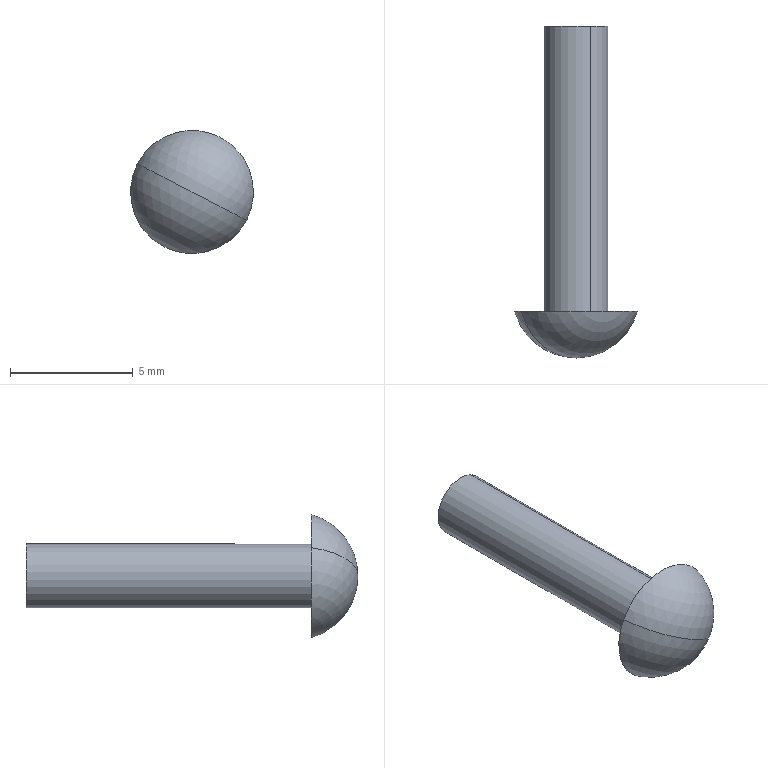Part | SolidWorks | features BaseBody 1 | 1 solid | 6 faces | box 5 x 13.501 x 5 mm | volume 83.832 mm3 | sphere 2 | plane 2 | cylinder 2 | commonest cylinder face diameters 2.6 x2
STEP:
#1=CARTESIAN_POINT('',(-214.693,5.922,3.237));
#2=VERTEX_POINT('',#1);
#3=CARTESIAN_POINT('',(-210.253,5.923,0.9371));
#4=VERTEX_POINT('',#3);
#5=CARTESIAN_POINT('',(-212.473,6.618,2.087));
#6=DIRECTION('',(0.46,-0.0003779,0.8879));
#7=DIRECTION('',(0.00003827,-1.,-0.0004455));
#8=AXIS2_PLACEMENT_3D('',#5,#6,#7);
#9=CIRCLE('',#8,2.595);
#10=EDGE_CURVE('',#2,#4,#9,.T.);
#11=ORIENTED_EDGE('',*,*,#10,.F.);
#12=CARTESIAN_POINT('',(-212.473,5.923,2.087));
#13=DIRECTION('',(-0.00003827,1.,0.0004455));
#14=DIRECTION('',(0.8879,0.0002389,-0.46));
#15=AXIS2_PLACEMENT_3D('',#12,#13,#14);
#16=CIRCLE('',#15,2.5);
#17=EDGE_CURVE('',#4,#2,#16,.T.);
#18=ORIENTED_EDGE('',*,*,#17,.F.);
#19=EDGE_LOOP('',(#11,#18));
#20=FACE_OUTER_BOUND('',#19,.T.);
#21=CARTESIAN_POINT('',(-212.473,6.618,2.087));
#22=DIRECTION('',(0.46,-0.0003779,0.8879));
#23=DIRECTION('',(-0.8879,-0.0002389,0.46));
#24=AXIS2_PLACEMENT_3D('',#21,#22,#23);
#25=SPHERICAL_SURFACE('',#24,2.595);
#26=ADVANCED_FACE('',(#20),#25,.T.);
#27=CARTESIAN_POINT('',(-213.071,5.923,0.9327));
#28=VERTEX_POINT('',#27);
#29=CARTESIAN_POINT('',(-211.875,5.922,3.241));
#30=VERTEX_POINT('',#29);
#31=CARTESIAN_POINT('',(-212.473,5.923,2.087));
#32=DIRECTION('',(-0.00003827,1.,0.0004455));
#33=DIRECTION('',(-0.46,0.0003779,-0.8879));
#34=AXIS2_PLACEMENT_3D('',#31,#32,#33);
#35=CIRCLE('',#34,1.3);
#36=EDGE_CURVE('',#28,#30,#35,.T.);
#37=ORIENTED_EDGE('',*,*,#36,.F.);
#38=CARTESIAN_POINT('',(-212.473,5.923,2.087));
#39=DIRECTION('',(-0.00003827,1.,0.0004455));
#40=DIRECTION('',(0.46,-0.0003779,0.8879));
#41=AXIS2_PLACEMENT_3D('',#38,#39,#40);
#42=CIRCLE('',#41,1.3);
#43=EDGE_CURVE('',#30,#28,#42,.T.);
#44=ORIENTED_EDGE('',*,*,#43,.F.);
#45=EDGE_LOOP('',(#37,#44));
#46=FACE_BOUND('',#45,.T.);
#47=CARTESIAN_POINT('',(-212.473,5.923,2.087));
#48=DIRECTION('',(-0.00003827,1.,0.0004455));
#49=DIRECTION('',(-0.8879,-0.0002389,0.46));
#50=AXIS2_PLACEMENT_3D('',#47,#48,#49);
#51=CIRCLE('',#50,2.5);
#52=EDGE_CURVE('',#2,#4,#51,.T.);
#53=ORIENTED_EDGE('',*,*,#52,.T.);
#54=ORIENTED_EDGE('',*,*,#17,.T.);
#55=EDGE_LOOP('',(#53,#54));
#56=FACE_OUTER_BOUND('',#55,.T.);
#57=CARTESIAN_POINT('',(-211.319,5.923,1.489));
#58=DIRECTION('',(-0.00003827,1.,0.0004455));
#59=DIRECTION('',(0.9963,0.,0.08559));
#60=AXIS2_PLACEMENT_3D('',#57,#58,#59);
#61=PLANE('',#60);
#62=ADVANCED_FACE('',(#46,#56),#61,.T.);
#63=ORIENTED_EDGE('',*,*,#10,.T.);
#64=ORIENTED_EDGE('',*,*,#52,.F.);
#65=EDGE_LOOP('',(#63,#64));
#66=FACE_OUTER_BOUND('',#65,.T.);
#67=CARTESIAN_POINT('',(-212.473,6.618,2.087));
#68=DIRECTION('',(0.46,-0.0003779,0.8879));
#69=DIRECTION('',(-0.8879,-0.0002389,0.46));
#70=AXIS2_PLACEMENT_3D('',#67,#68,#69);
#71=SPHERICAL_SURFACE('',#70,2.595);
#72=ADVANCED_FACE('',(#66),#71,.T.);
#73=CARTESIAN_POINT('',(-211.875,17.522,3.246));
#74=VERTEX_POINT('',#73);
#75=CARTESIAN_POINT('',(-211.875,5.922,3.241));
#76=DIRECTION('',(-0.00003827,1.,0.0004455));
#77=VECTOR('',#76,1000.);
#78=LINE('',#75,#77);
#79=EDGE_CURVE('',#30,#74,#78,.T.);
#80=ORIENTED_EDGE('',*,*,#79,.F.);
#81=ORIENTED_EDGE('',*,*,#43,.T.);
#82=CARTESIAN_POINT('',(-213.071,17.523,0.9379));
#83=VERTEX_POINT('',#82);
#84=CARTESIAN_POINT('',(-213.071,5.923,0.9327));
#85=DIRECTION('',(-0.00003827,1.,0.0004455));
#86=VECTOR('',#85,1000.);
#87=LINE('',#84,#86);
#88=EDGE_CURVE('',#28,#83,#87,.T.);
#89=ORIENTED_EDGE('',*,*,#88,.T.);
#90=CARTESIAN_POINT('',(-212.473,17.523,2.092));
#91=DIRECTION('',(0.00003827,-1.,-0.0004455));
#92=DIRECTION('',(-0.46,0.0003779,-0.8879));
#93=AXIS2_PLACEMENT_3D('',#90,#91,#92);
#94=CIRCLE('',#93,1.3);
#95=EDGE_CURVE('',#83,#74,#94,.T.);
#96=ORIENTED_EDGE('',*,*,#95,.T.);
#97=EDGE_LOOP('',(#80,#81,#89,#96));
#98=FACE_OUTER_BOUND('',#97,.T.);
#99=CARTESIAN_POINT('',(-212.473,4.023,2.086));
#100=DIRECTION('',(0.00003827,-1.,-0.0004455));
#101=DIRECTION('',(-0.46,0.0003779,-0.8879));
#102=AXIS2_PLACEMENT_3D('',#99,#100,#101);
#103=CYLINDRICAL_SURFACE('',#102,1.3);
#104=ADVANCED_FACE('',(#98),#103,.T.);
#105=CARTESIAN_POINT('',(-212.473,17.523,2.092));
#106=DIRECTION('',(0.00003827,-1.,-0.0004455));
#107=DIRECTION('',(0.46,-0.0003779,0.8879));
#108=AXIS2_PLACEMENT_3D('',#105,#106,#107);
#109=CIRCLE('',#108,1.3);
#110=EDGE_CURVE('',#74,#83,#109,.T.);
#111=ORIENTED_EDGE('',*,*,#110,.F.);
#112=ORIENTED_EDGE('',*,*,#95,.F.);
#113=EDGE_LOOP('',(#111,#112));
#114=FACE_OUTER_BOUND('',#113,.T.);
#115=CARTESIAN_POINT('',(-212.473,17.523,2.092));
#116=DIRECTION('',(-0.00003827,1.,0.0004455));
#117=DIRECTION('',(0.9963,0.,0.08559));
#118=AXIS2_PLACEMENT_3D('',#115,#116,#117);
#119=PLANE('',#118);
#120=ADVANCED_FACE('',(#114),#119,.T.);
#121=ORIENTED_EDGE('',*,*,#110,.T.);
#122=ORIENTED_EDGE('',*,*,#88,.F.);
#123=ORIENTED_EDGE('',*,*,#36,.T.);
#124=ORIENTED_EDGE('',*,*,#79,.T.);
#125=EDGE_LOOP('',(#121,#122,#123,#124));
#126=FACE_OUTER_BOUND('',#125,.T.);
#127=CARTESIAN_POINT('',(-212.473,4.023,2.086));
#128=DIRECTION('',(0.00003827,-1.,-0.0004455));
#129=DIRECTION('',(-0.46,0.0003779,-0.8879));
#130=AXIS2_PLACEMENT_3D('',#127,#128,#129);
#131=CYLINDRICAL_SURFACE('',#130,1.3);
#132=ADVANCED_FACE('',(#126),#131,.T.);
#133=CLOSED_SHELL('',(#26,#62,#72,#104,#120,#132));
#134=MANIFOLD_SOLID_BREP('',#133);
#135=CARTESIAN_POINT('',(0.,0.,0.));
#136=DIRECTION('',(0.,0.,1.));
#137=DIRECTION('',(1.,0.,0.));
#138=AXIS2_PLACEMENT_3D('',#135,#136,#137);
#139=(LENGTH_UNIT()NAMED_UNIT(*)SI_UNIT(.MILLI.,.METRE.));
#140=UNCERTAINTY_MEASURE_WITH_UNIT(LENGTH_MEASURE(0.00001),#139,'','');
#141=(NAMED_UNIT(*)PLANE_ANGLE_UNIT()SI_UNIT($,.RADIAN.));
#142=(NAMED_UNIT(*)SI_UNIT($,.STERADIAN.)SOLID_ANGLE_UNIT());
#143=(GEOMETRIC_REPRESENTATION_CONTEXT(3)GLOBAL_UNCERTAINTY_ASSIGNED_CONTEXT((#140))GLOBAL_UNIT_ASSIGNED_CONTEXT((#139,#141,#142))REPRESENTATION_CONTEXT('',''));
#144=ADVANCED_BREP_SHAPE_REPRESENTATION('',(#134,#138),#143);